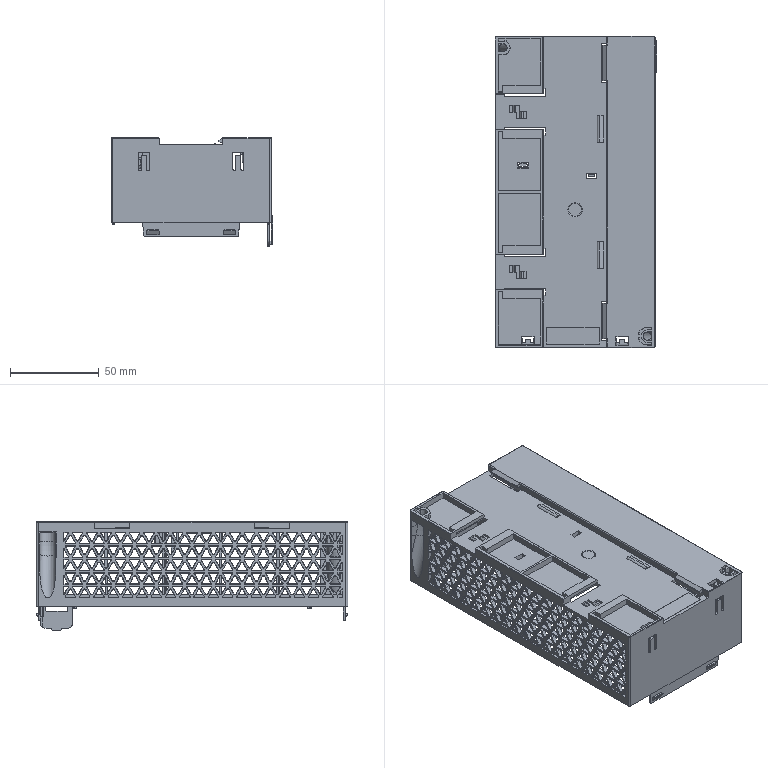Part | Creo | 1 solid | 3976 faces | volume 76458 mm3 | spline 1542 | plane 1347 | cone 823 | cylinder 230 | torus 20 | sphere 10 | other 4 | commonest cylinder face diameters 0.603 x77 0.402 x58 1.005 x41 2.01 x14 5.025 x4 5.226 x4